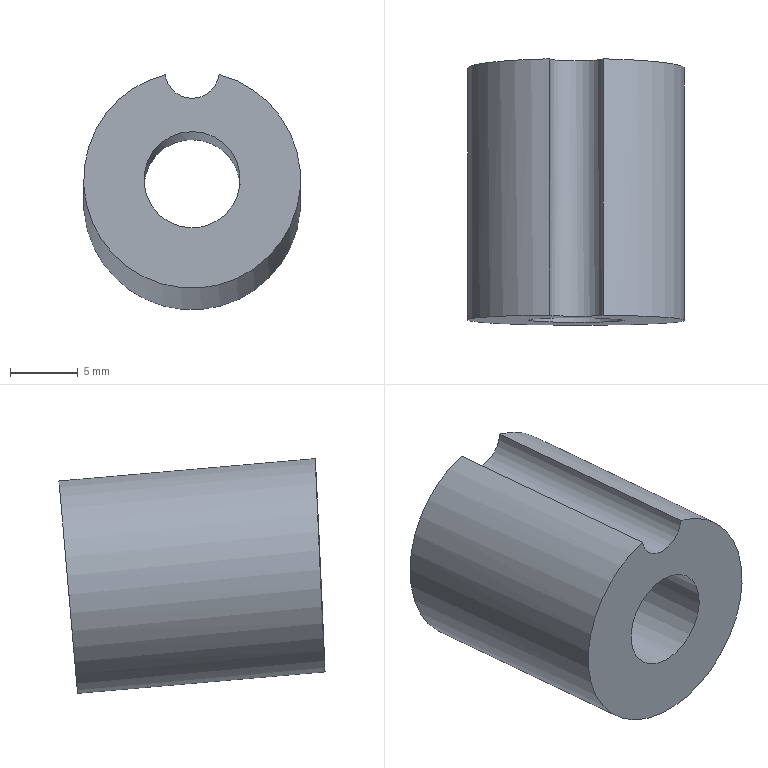Part | NX | features EKSD 16-20-7.100 2 | 1 solid | 7 faces | box 16 x 19.62 x 17.344 mm | volume 2315 mm3 | cylinder 4 | plane 3 | commonest cylinder face diameters 4 x1 7.1 x1 10.6 x1 16 x1
STEP:
#1=CARTESIAN_POINT('',(77.644,-27.171,-37.258));
#2=VERTEX_POINT('',#1);
#3=CARTESIAN_POINT('',(81.613,-27.171,-37.258));
#4=VERTEX_POINT('',#3);
#5=CARTESIAN_POINT('',(79.629,-27.149,-37.009));
#6=DIRECTION('',(0.,-0.9962,0.08716));
#7=DIRECTION('',(0.,-0.08716,-0.9962));
#8=AXIS2_PLACEMENT_3D('',#5,#6,#7);
#9=CIRCLE('',#8,2.);
#10=EDGE_CURVE('',#2,#4,#9,.T.);
#11=ORIENTED_EDGE('',*,*,#10,.T.);
#12=CARTESIAN_POINT('',(79.629,-27.846,-44.978));
#13=DIRECTION('',(0.,-0.9962,0.08716));
#14=DIRECTION('',(0.,-0.08716,-0.9962));
#15=AXIS2_PLACEMENT_3D('',#12,#13,#14);
#16=CIRCLE('',#15,8.);
#17=EDGE_CURVE('',#2,#4,#16,.T.);
#18=ORIENTED_EDGE('',*,*,#17,.F.);
#19=EDGE_LOOP('',(#11,#18));
#20=FACE_BOUND('',#19,.T.);
#21=CARTESIAN_POINT('',(79.629,-27.384,-39.698));
#22=VERTEX_POINT('',#21);
#23=CARTESIAN_POINT('',(79.629,-27.846,-44.978));
#24=DIRECTION('',(0.,0.9962,-0.08716));
#25=DIRECTION('',(0.,0.08716,0.9962));
#26=AXIS2_PLACEMENT_3D('',#23,#24,#25);
#27=CIRCLE('',#26,5.3);
#28=EDGE_CURVE('',#22,#22,#27,.T.);
#29=ORIENTED_EDGE('',*,*,#28,.F.);
#30=EDGE_LOOP('',(#29));
#31=FACE_BOUND('',#30,.T.);
#32=CARTESIAN_POINT('',(79.629,-27.846,-44.978));
#33=DIRECTION('',(0.,0.9962,-0.08716));
#34=DIRECTION('',(0.,0.08716,0.9962));
#35=AXIS2_PLACEMENT_3D('',#32,#33,#34);
#36=PLANE('',#35);
#37=ADVANCED_FACE('',(#20,#31),#36,.T.);
#38=CARTESIAN_POINT('',(81.613,-46.077,-35.604));
#39=VERTEX_POINT('',#38);
#40=CARTESIAN_POINT('',(77.644,-46.07,-35.604));
#41=VERTEX_POINT('',#40);
#42=CARTESIAN_POINT('',(79.629,-46.062,-35.354));
#43=DIRECTION('',(0.001957,0.999,-0.04546));
#44=DIRECTION('',(-0.04675,-0.04532,-0.9979));
#45=AXIS2_PLACEMENT_3D('',#42,#43,#44);
#46=ELLIPSE('',#45,2.002,2.);
#47=EDGE_CURVE('',#39,#41,#46,.T.);
#48=ORIENTED_EDGE('',*,*,#47,.T.);
#49=CARTESIAN_POINT('',(79.629,-46.426,-43.353));
#50=DIRECTION('',(0.001957,0.999,-0.04546));
#51=DIRECTION('',(-0.04675,-0.04532,-0.9979));
#52=AXIS2_PLACEMENT_3D('',#49,#50,#51);
#53=ELLIPSE('',#52,8.007,8.);
#54=EDGE_CURVE('',#39,#41,#53,.T.);
#55=ORIENTED_EDGE('',*,*,#54,.F.);
#56=EDGE_LOOP('',(#48,#55));
#57=FACE_BOUND('',#56,.T.);
#58=CARTESIAN_POINT('',(79.463,-46.587,-46.898));
#59=VERTEX_POINT('',#58);
#60=CARTESIAN_POINT('',(79.629,-46.426,-43.353));
#61=DIRECTION('',(0.001957,0.999,-0.04546));
#62=DIRECTION('',(-0.04675,-0.04532,-0.9979));
#63=AXIS2_PLACEMENT_3D('',#60,#61,#62);
#64=ELLIPSE('',#63,3.553,3.55);
#65=EDGE_CURVE('',#59,#59,#64,.F.);
#66=ORIENTED_EDGE('',*,*,#65,.F.);
#67=EDGE_LOOP('',(#66));
#68=FACE_BOUND('',#67,.T.);
#69=CARTESIAN_POINT('',(128.811,-48.589,-88.763));
#70=DIRECTION('',(0.001957,0.999,-0.04546));
#71=DIRECTION('',(0.06617,0.04523,0.9968));
#72=AXIS2_PLACEMENT_3D('',#69,#70,#71);
#73=PLANE('',#72);
#74=ADVANCED_FACE('',(#57,#68),#73,.F.);
#75=CARTESIAN_POINT('',(81.613,-37.133,-36.386));
#76=DIRECTION('',(0.,0.9962,-0.08716));
#77=VECTOR('',#76,1000.);
#78=LINE('',#75,#77);
#79=EDGE_CURVE('',#39,#4,#78,.T.);
#80=ORIENTED_EDGE('',*,*,#79,.F.);
#81=ORIENTED_EDGE('',*,*,#54,.T.);
#82=CARTESIAN_POINT('',(77.644,-37.133,-36.386));
#83=DIRECTION('',(0.,0.9962,-0.08716));
#84=VECTOR('',#83,1000.);
#85=LINE('',#82,#84);
#86=EDGE_CURVE('',#2,#41,#85,.F.);
#87=ORIENTED_EDGE('',*,*,#86,.F.);
#88=ORIENTED_EDGE('',*,*,#17,.T.);
#89=EDGE_LOOP('',(#80,#81,#87,#88));
#90=FACE_BOUND('',#89,.T.);
#91=CARTESIAN_POINT('',(79.629,-47.77,-43.235));
#92=DIRECTION('',(0.,0.9962,-0.08716));
#93=DIRECTION('',(0.,0.08716,0.9962));
#94=AXIS2_PLACEMENT_3D('',#91,#92,#93);
#95=CYLINDRICAL_SURFACE('',#94,8.);
#96=ADVANCED_FACE('',(#90),#95,.T.);
#97=CARTESIAN_POINT('',(79.629,-40.11,-47.469));
#98=VERTEX_POINT('',#97);
#99=CARTESIAN_POINT('',(79.629,-39.801,-43.932));
#100=DIRECTION('',(0.,-0.9962,0.08716));
#101=DIRECTION('',(0.,-0.08716,-0.9962));
#102=AXIS2_PLACEMENT_3D('',#99,#100,#101);
#103=CIRCLE('',#102,3.55);
#104=EDGE_CURVE('',#98,#98,#103,.F.);
#105=ORIENTED_EDGE('',*,*,#104,.T.);
#106=EDGE_LOOP('',(#105));
#107=FACE_BOUND('',#106,.T.);
#108=ORIENTED_EDGE('',*,*,#65,.T.);
#109=EDGE_LOOP('',(#108));
#110=FACE_BOUND('',#109,.T.);
#111=CARTESIAN_POINT('',(79.629,-48.766,-43.148));
#112=DIRECTION('',(0.,0.9962,-0.08716));
#113=DIRECTION('',(0.,0.08716,0.9962));
#114=AXIS2_PLACEMENT_3D('',#111,#112,#113);
#115=CYLINDRICAL_SURFACE('',#114,3.55);
#116=ADVANCED_FACE('',(#107,#110),#115,.F.);
#117=CARTESIAN_POINT('',(79.629,-39.339,-38.652));
#118=VERTEX_POINT('',#117);
#119=CARTESIAN_POINT('',(79.629,-39.801,-43.932));
#120=DIRECTION('',(0.,0.9962,-0.08716));
#121=DIRECTION('',(0.,0.08716,0.9962));
#122=AXIS2_PLACEMENT_3D('',#119,#120,#121);
#123=CIRCLE('',#122,5.3);
#124=EDGE_CURVE('',#118,#118,#123,.T.);
#125=ORIENTED_EDGE('',*,*,#124,.T.);
#126=EDGE_LOOP('',(#125));
#127=FACE_BOUND('',#126,.T.);
#128=ORIENTED_EDGE('',*,*,#104,.F.);
#129=EDGE_LOOP('',(#128));
#130=FACE_BOUND('',#129,.T.);
#131=CARTESIAN_POINT('',(79.629,-39.801,-43.932));
#132=DIRECTION('',(0.,-0.9962,0.08716));
#133=DIRECTION('',(0.,-0.08716,-0.9962));
#134=AXIS2_PLACEMENT_3D('',#131,#132,#133);
#135=PLANE('',#134);
#136=ADVANCED_FACE('',(#127,#130),#135,.F.);
#137=ORIENTED_EDGE('',*,*,#28,.T.);
#138=EDGE_LOOP('',(#137));
#139=FACE_BOUND('',#138,.T.);
#140=ORIENTED_EDGE('',*,*,#124,.F.);
#141=EDGE_LOOP('',(#140));
#142=FACE_BOUND('',#141,.T.);
#143=CARTESIAN_POINT('',(79.629,-39.801,-43.932));
#144=DIRECTION('',(0.,0.9962,-0.08716));
#145=DIRECTION('',(0.,0.08716,0.9962));
#146=AXIS2_PLACEMENT_3D('',#143,#144,#145);
#147=CYLINDRICAL_SURFACE('',#146,5.3);
#148=ADVANCED_FACE('',(#139,#142),#147,.F.);
#149=ORIENTED_EDGE('',*,*,#79,.T.);
#150=ORIENTED_EDGE('',*,*,#10,.F.);
#151=ORIENTED_EDGE('',*,*,#86,.T.);
#152=ORIENTED_EDGE('',*,*,#47,.F.);
#153=EDGE_LOOP('',(#149,#150,#151,#152));
#154=FACE_BOUND('',#153,.T.);
#155=CARTESIAN_POINT('',(79.629,-47.073,-35.266));
#156=DIRECTION('',(0.,0.9962,-0.08716));
#157=DIRECTION('',(0.,0.08716,0.9962));
#158=AXIS2_PLACEMENT_3D('',#155,#156,#157);
#159=CYLINDRICAL_SURFACE('',#158,2.);
#160=ADVANCED_FACE('',(#154),#159,.F.);
#161=CLOSED_SHELL('',(#37,#74,#96,#116,#136,#148,#160));
#162=MANIFOLD_SOLID_BREP('',#161);
#163=(LENGTH_UNIT()NAMED_UNIT(*)SI_UNIT(.MILLI.,.METRE.));
#164=UNCERTAINTY_MEASURE_WITH_UNIT(LENGTH_MEASURE(0.00001),#163,'','');
#165=(NAMED_UNIT(*)PLANE_ANGLE_UNIT()SI_UNIT($,.RADIAN.));
#166=(NAMED_UNIT(*)SI_UNIT($,.STERADIAN.)SOLID_ANGLE_UNIT());
#167=(GEOMETRIC_REPRESENTATION_CONTEXT(3)GLOBAL_UNCERTAINTY_ASSIGNED_CONTEXT((#164))GLOBAL_UNIT_ASSIGNED_CONTEXT((#163,#165,#166))REPRESENTATION_CONTEXT('',''));
#168=ADVANCED_BREP_SHAPE_REPRESENTATION('',(#162),#167);